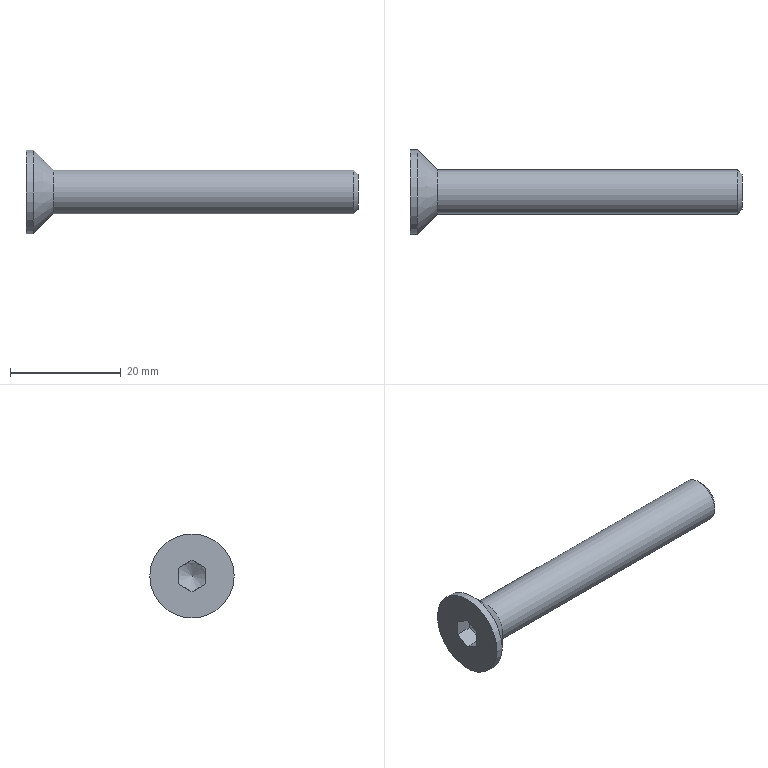Part | STEP file | DIN 7991 - M8  x  60 | 1 solid | 13 faces | box 60 x 15.24 x 15.24 mm | volume 3321 mm3 | plane 8 | cone 3 | cylinder 2 | commonest cylinder face diameters 8 x1 15.24 x1
STEP:
#1=CARTESIAN_POINT('',(0.,0.,0.));
#2=DIRECTION('',(0.,0.,1.));
#3=DIRECTION('',(1.,0.,0.));
#4=AXIS2_PLACEMENT_3D('',#1,#2,#3);
#5=CARTESIAN_POINT('',(59.233,4.,0.));
#6=VERTEX_POINT('',#5);
#7=CARTESIAN_POINT('',(59.233,0.,0.));
#8=DIRECTION('',(1.,0.,0.));
#9=DIRECTION('',(0.,-1.,0.));
#10=AXIS2_PLACEMENT_3D('',#7,#8,#9);
#11=CIRCLE('',#10,4.);
#12=CARTESIAN_POINT('',(59.617,0.,0.));
#13=DIRECTION('',(-1.,0.,0.));
#14=DIRECTION('',(0.,-1.,0.));
#15=AXIS2_PLACEMENT_3D('',#12,#13,#14);
#16=CONICAL_SURFACE('',#15,3.617,0.7854);
#17=CARTESIAN_POINT('',(12.566,0.3834));
#18=DIRECTION('',(-1.,0.));
#19=VECTOR('',#18,1.);
#20=LINE('',#17,#19);
#21=(GEOMETRIC_REPRESENTATION_CONTEXT(2)PARAMETRIC_REPRESENTATION_CONTEXT()REPRESENTATION_CONTEXT('',''));
#22=DEFINITIONAL_REPRESENTATION('',(#20),#21);
#23=PCURVE('',#16,#22);
#24=CARTESIAN_POINT('',(46.,0.,0.));
#25=DIRECTION('',(1.,0.,0.));
#26=DIRECTION('',(0.,1.,0.));
#27=AXIS2_PLACEMENT_3D('',#24,#25,#26);
#28=CYLINDRICAL_SURFACE('',#27,4.);
#29=CARTESIAN_POINT('',(-3.142,13.233));
#30=DIRECTION('',(1.,0.));
#31=VECTOR('',#30,1.);
#32=LINE('',#29,#31);
#33=(GEOMETRIC_REPRESENTATION_CONTEXT(2)PARAMETRIC_REPRESENTATION_CONTEXT()REPRESENTATION_CONTEXT('',''));
#34=DEFINITIONAL_REPRESENTATION('',(#32),#33);
#35=PCURVE('',#28,#34);
#36=SURFACE_CURVE('',#11,(#23,#35),.PCURVE_S1.);
#37=EDGE_CURVE('',#6,#6,#36,.T.);
#38=ORIENTED_EDGE('',*,*,#37,.T.);
#39=CARTESIAN_POINT('',(60.,3.233,0.));
#40=VERTEX_POINT('',#39);
#41=CARTESIAN_POINT('',(60.,3.233,0.));
#42=CARTESIAN_POINT('',(59.233,4.,0.));
#43=B_SPLINE_CURVE_WITH_KNOTS('',1,(#41,#42),.UNSPECIFIED.,.F.,.F.,(2,2),(-0.5422,0.5422),.PIECEWISE_BEZIER_KNOTS.);
#44=CARTESIAN_POINT('',(3.142,0.));
#45=DIRECTION('',(0.,1.));
#46=VECTOR('',#45,1.);
#47=LINE('',#44,#46);
#48=(GEOMETRIC_REPRESENTATION_CONTEXT(2)PARAMETRIC_REPRESENTATION_CONTEXT()REPRESENTATION_CONTEXT('',''));
#49=DEFINITIONAL_REPRESENTATION('',(#47),#48);
#50=PCURVE('',#16,#49);
#51=CARTESIAN_POINT('',(9.425,0.));
#52=DIRECTION('',(0.,1.));
#53=VECTOR('',#52,1.);
#54=LINE('',#51,#53);
#55=(GEOMETRIC_REPRESENTATION_CONTEXT(2)PARAMETRIC_REPRESENTATION_CONTEXT()REPRESENTATION_CONTEXT('',''));
#56=DEFINITIONAL_REPRESENTATION('',(#54),#55);
#57=PCURVE('',#16,#56);
#58=SEAM_CURVE('',#43,(#50,#57),.PCURVE_S1.);
#59=EDGE_CURVE('',#40,#6,#58,.T.);
#60=ORIENTED_EDGE('',*,*,#59,.F.);
#61=CARTESIAN_POINT('',(60.,0.,0.));
#62=DIRECTION('',(-1.,0.,0.));
#63=DIRECTION('',(0.,-1.,0.));
#64=AXIS2_PLACEMENT_3D('',#61,#62,#63);
#65=CIRCLE('',#64,3.233);
#66=CARTESIAN_POINT('',(0.,-0.3834));
#67=DIRECTION('',(1.,0.));
#68=VECTOR('',#67,1.);
#69=LINE('',#66,#68);
#70=(GEOMETRIC_REPRESENTATION_CONTEXT(2)PARAMETRIC_REPRESENTATION_CONTEXT()REPRESENTATION_CONTEXT('',''));
#71=DEFINITIONAL_REPRESENTATION('',(#69),#70);
#72=PCURVE('',#16,#71);
#73=CARTESIAN_POINT('',(60.,2.,0.));
#74=DIRECTION('',(1.,0.,0.));
#75=DIRECTION('',(0.,0.,-1.));
#76=AXIS2_PLACEMENT_3D('',#73,#74,#75);
#77=PLANE('',#76);
#78=CARTESIAN_POINT('',(0.,-5.233));
#79=CARTESIAN_POINT('',(-5.6,-5.233));
#80=CARTESIAN_POINT('',(-2.8,-0.3834));
#81=CARTESIAN_POINT('',(0.,4.466));
#82=CARTESIAN_POINT('',(2.8,-0.3834));
#83=CARTESIAN_POINT('',(5.6,-5.233));
#84=CARTESIAN_POINT('',(0.,-5.233));
#85=(BOUNDED_CURVE()B_SPLINE_CURVE(2,(#78,#79,#80,#81,#82,#83,#84),.UNSPECIFIED.,.T.,.F.)B_SPLINE_CURVE_WITH_KNOTS((1,2,2,2,2,1),(-2.094,0.,2.094,4.189,6.283,8.378),.UNSPECIFIED.)CURVE()GEOMETRIC_REPRESENTATION_ITEM()RATIONAL_B_SPLINE_CURVE((1.,0.5,1.,0.5,1.,0.5,1.))REPRESENTATION_ITEM(''));
#86=(GEOMETRIC_REPRESENTATION_CONTEXT(2)PARAMETRIC_REPRESENTATION_CONTEXT()REPRESENTATION_CONTEXT('',''));
#87=DEFINITIONAL_REPRESENTATION('',(#85),#86);
#88=PCURVE('',#77,#87);
#89=SURFACE_CURVE('',#65,(#72,#88),.PCURVE_S1.);
#90=EDGE_CURVE('',#40,#40,#89,.T.);
#91=ORIENTED_EDGE('',*,*,#90,.T.);
#92=ORIENTED_EDGE('',*,*,#59,.T.);
#93=EDGE_LOOP('',(#38,#60,#91,#92));
#94=FACE_BOUND('',#93,.T.);
#95=ADVANCED_FACE('',(#94),#16,.T.);
#96=CARTESIAN_POINT('',(4.96,4.,0.));
#97=VERTEX_POINT('',#96);
#98=CARTESIAN_POINT('',(4.96,0.,0.));
#99=DIRECTION('',(1.,0.,0.));
#100=DIRECTION('',(0.,1.,0.));
#101=AXIS2_PLACEMENT_3D('',#98,#99,#100);
#102=CIRCLE('',#101,4.);
#103=CARTESIAN_POINT('',(0.,-41.04));
#104=DIRECTION('',(1.,0.));
#105=VECTOR('',#104,1.);
#106=LINE('',#103,#105);
#107=(GEOMETRIC_REPRESENTATION_CONTEXT(2)PARAMETRIC_REPRESENTATION_CONTEXT()REPRESENTATION_CONTEXT('',''));
#108=DEFINITIONAL_REPRESENTATION('',(#106),#107);
#109=PCURVE('',#28,#108);
#110=CARTESIAN_POINT('',(3.15,0.,0.));
#111=DIRECTION('',(-1.,0.,0.));
#112=DIRECTION('',(0.,1.,0.));
#113=AXIS2_PLACEMENT_3D('',#110,#111,#112);
#114=CONICAL_SURFACE('',#113,5.81,0.7854);
#115=CARTESIAN_POINT('',(6.283,-1.81));
#116=DIRECTION('',(-1.,0.));
#117=VECTOR('',#116,1.);
#118=LINE('',#115,#117);
#119=(GEOMETRIC_REPRESENTATION_CONTEXT(2)PARAMETRIC_REPRESENTATION_CONTEXT()REPRESENTATION_CONTEXT('',''));
#120=DEFINITIONAL_REPRESENTATION('',(#118),#119);
#121=PCURVE('',#114,#120);
#122=SURFACE_CURVE('',#102,(#109,#121),.PCURVE_S1.);
#123=EDGE_CURVE('',#97,#97,#122,.T.);
#124=ORIENTED_EDGE('',*,*,#123,.T.);
#125=CARTESIAN_POINT('',(4.96,4.,0.));
#126=CARTESIAN_POINT('',(59.233,4.,0.));
#127=B_SPLINE_CURVE_WITH_KNOTS('',1,(#125,#126),.UNSPECIFIED.,.F.,.F.,(2,2),(-41.04,13.233),.PIECEWISE_BEZIER_KNOTS.);
#128=CARTESIAN_POINT('',(6.283,0.));
#129=DIRECTION('',(0.,1.));
#130=VECTOR('',#129,1.);
#131=LINE('',#128,#130);
#132=(GEOMETRIC_REPRESENTATION_CONTEXT(2)PARAMETRIC_REPRESENTATION_CONTEXT()REPRESENTATION_CONTEXT('',''));
#133=DEFINITIONAL_REPRESENTATION('',(#131),#132);
#134=PCURVE('',#28,#133);
#135=CARTESIAN_POINT('',(0.,0.));
#136=DIRECTION('',(0.,1.));
#137=VECTOR('',#136,1.);
#138=LINE('',#135,#137);
#139=(GEOMETRIC_REPRESENTATION_CONTEXT(2)PARAMETRIC_REPRESENTATION_CONTEXT()REPRESENTATION_CONTEXT('',''));
#140=DEFINITIONAL_REPRESENTATION('',(#138),#139);
#141=PCURVE('',#28,#140);
#142=SEAM_CURVE('',#127,(#134,#141),.PCURVE_S1.);
#143=EDGE_CURVE('',#97,#6,#142,.T.);
#144=ORIENTED_EDGE('',*,*,#143,.T.);
#145=ORIENTED_EDGE('',*,*,#37,.F.);
#146=ORIENTED_EDGE('',*,*,#143,.F.);
#147=EDGE_LOOP('',(#124,#144,#145,#146));
#148=FACE_BOUND('',#147,.T.);
#149=ADVANCED_FACE('',(#148),#28,.T.);
#150=ORIENTED_EDGE('',*,*,#90,.F.);
#151=EDGE_LOOP('',(#150));
#152=FACE_BOUND('',#151,.T.);
#153=ADVANCED_FACE('',(#152),#77,.T.);
#154=CARTESIAN_POINT('',(3.,-2.5,-1.443));
#155=VERTEX_POINT('',#154);
#156=CARTESIAN_POINT('',(3.,-2.5,1.443));
#157=VERTEX_POINT('',#156);
#158=CARTESIAN_POINT('',(3.,-2.5,-1.443));
#159=CARTESIAN_POINT('',(3.417,-2.5,0.));
#160=CARTESIAN_POINT('',(3.,-2.5,1.443));
#161=(BOUNDED_CURVE()B_SPLINE_CURVE(2,(#158,#159,#160),.UNSPECIFIED.,.F.,.F.)B_SPLINE_CURVE_WITH_KNOTS((3,3),(0.,0.2921),.PIECEWISE_BEZIER_KNOTS.)CURVE()GEOMETRIC_REPRESENTATION_ITEM()RATIONAL_B_SPLINE_CURVE((1.,1.155,1.))REPRESENTATION_ITEM(''));
#162=CARTESIAN_POINT('',(0.,-2.5,-1.443));
#163=DIRECTION('',(0.,-1.,0.));
#164=DIRECTION('',(0.,0.,-1.));
#165=AXIS2_PLACEMENT_3D('',#162,#163,#164);
#166=PLANE('',#165);
#167=CARTESIAN_POINT('',(0.,3.));
#168=CARTESIAN_POINT('',(-1.443,3.417));
#169=CARTESIAN_POINT('',(-2.887,3.));
#170=(BOUNDED_CURVE()B_SPLINE_CURVE(2,(#167,#168,#169),.UNSPECIFIED.,.F.,.F.)B_SPLINE_CURVE_WITH_KNOTS((3,3),(0.,0.2921),.PIECEWISE_BEZIER_KNOTS.)CURVE()GEOMETRIC_REPRESENTATION_ITEM()RATIONAL_B_SPLINE_CURVE((1.,1.155,1.))REPRESENTATION_ITEM(''));
#171=(GEOMETRIC_REPRESENTATION_CONTEXT(2)PARAMETRIC_REPRESENTATION_CONTEXT()REPRESENTATION_CONTEXT('',''));
#172=DEFINITIONAL_REPRESENTATION('',(#170),#171);
#173=PCURVE('',#166,#172);
#174=CARTESIAN_POINT('',(3.833,0.,0.));
#175=DIRECTION('',(-1.,0.,0.));
#176=DIRECTION('',(0.,1.,0.));
#177=AXIS2_PLACEMENT_3D('',#174,#175,#176);
#178=CONICAL_SURFACE('',#177,1.443,1.047);
#179=CARTESIAN_POINT('',(8.901,0.8333));
#180=CARTESIAN_POINT('',(8.916,0.8188));
#181=CARTESIAN_POINT('',(8.947,0.7913));
#182=CARTESIAN_POINT('',(8.993,0.755));
#183=CARTESIAN_POINT('',(9.04,0.7233));
#184=CARTESIAN_POINT('',(9.087,0.6958));
#185=CARTESIAN_POINT('',(9.134,0.6724));
#186=CARTESIAN_POINT('',(9.182,0.6529));
#187=CARTESIAN_POINT('',(9.23,0.6371));
#188=CARTESIAN_POINT('',(9.279,0.625));
#189=CARTESIAN_POINT('',(9.327,0.6163));
#190=CARTESIAN_POINT('',(9.376,0.6112));
#191=CARTESIAN_POINT('',(9.425,0.6095));
#192=CARTESIAN_POINT('',(9.473,0.6112));
#193=CARTESIAN_POINT('',(9.522,0.6163));
#194=CARTESIAN_POINT('',(9.571,0.625));
#195=CARTESIAN_POINT('',(9.619,0.6371));
#196=CARTESIAN_POINT('',(9.667,0.6529));
#197=CARTESIAN_POINT('',(9.715,0.6724));
#198=CARTESIAN_POINT('',(9.763,0.6958));
#199=CARTESIAN_POINT('',(9.81,0.7233));
#200=CARTESIAN_POINT('',(9.856,0.755));
#201=CARTESIAN_POINT('',(9.903,0.7913));
#202=CARTESIAN_POINT('',(9.933,0.8188));
#203=CARTESIAN_POINT('',(9.948,0.8333));
#204=B_SPLINE_CURVE_WITH_KNOTS('',3,(#179,#180,#181,#182,#183,#184,#185,#186,#187,#188,#189,#190,#191,#192,#193,#194,#195,#196,#197,#198,#199,#200,#201,#202,#203),.UNSPECIFIED.,.F.,.F.,(4,1,1,1,1,1,1,1,1,1,1,1,1,1,1,1,1,1,1,1,1,1,4),(0.,0.01328,0.02656,0.03983,0.05311,0.06639,0.07967,0.09294,0.1062,0.1195,0.1328,0.1461,0.1593,0.1726,0.1859,0.1992,0.2124,0.2257,0.239,0.2523,0.2656,0.2788,0.2921),.QUASI_UNIFORM_KNOTS.);
#205=(GEOMETRIC_REPRESENTATION_CONTEXT(2)PARAMETRIC_REPRESENTATION_CONTEXT()REPRESENTATION_CONTEXT('',''));
#206=DEFINITIONAL_REPRESENTATION('',(#204),#205);
#207=PCURVE('',#178,#206);
#208=SURFACE_CURVE('',#161,(#173,#207),.PCURVE_S1.);
#209=EDGE_CURVE('',#155,#157,#208,.T.);
#210=ORIENTED_EDGE('',*,*,#209,.F.);
#211=CARTESIAN_POINT('',(0.,-2.5,-1.443));
#212=VERTEX_POINT('',#211);
#213=CARTESIAN_POINT('',(1.5,-2.5,-1.443));
#214=DIRECTION('',(-1.,0.,0.));
#215=VECTOR('',#214,1.);
#216=LINE('',#213,#215);
#217=CARTESIAN_POINT('',(0.,1.5));
#218=DIRECTION('',(0.,-1.));
#219=VECTOR('',#218,1.);
#220=LINE('',#217,#219);
#221=(GEOMETRIC_REPRESENTATION_CONTEXT(2)PARAMETRIC_REPRESENTATION_CONTEXT()REPRESENTATION_CONTEXT('',''));
#222=DEFINITIONAL_REPRESENTATION('',(#220),#221);
#223=PCURVE('',#166,#222);
#224=CARTESIAN_POINT('',(0.,0.,-2.887));
#225=DIRECTION('',(0.,-0.5,-0.866));
#226=DIRECTION('',(-1.,0.,0.));
#227=AXIS2_PLACEMENT_3D('',#224,#225,#226);
#228=PLANE('',#227);
#229=CARTESIAN_POINT('',(-1.5,-2.887));
#230=DIRECTION('',(1.,0.));
#231=VECTOR('',#230,1.);
#232=LINE('',#229,#231);
#233=(GEOMETRIC_REPRESENTATION_CONTEXT(2)PARAMETRIC_REPRESENTATION_CONTEXT()REPRESENTATION_CONTEXT('',''));
#234=DEFINITIONAL_REPRESENTATION('',(#232),#233);
#235=PCURVE('',#228,#234);
#236=SURFACE_CURVE('',#216,(#223,#235),.PCURVE_S1.);
#237=EDGE_CURVE('',#155,#212,#236,.T.);
#238=ORIENTED_EDGE('',*,*,#237,.T.);
#239=CARTESIAN_POINT('',(0.,-2.5,1.443));
#240=VERTEX_POINT('',#239);
#241=CARTESIAN_POINT('',(0.,-2.5,-0.6526));
#242=DIRECTION('',(0.,0.,-1.));
#243=VECTOR('',#242,1.);
#244=LINE('',#241,#243);
#245=CARTESIAN_POINT('',(-0.7907,0.));
#246=DIRECTION('',(1.,0.));
#247=VECTOR('',#246,1.);
#248=LINE('',#245,#247);
#249=(GEOMETRIC_REPRESENTATION_CONTEXT(2)PARAMETRIC_REPRESENTATION_CONTEXT()REPRESENTATION_CONTEXT('',''));
#250=DEFINITIONAL_REPRESENTATION('',(#248),#249);
#251=PCURVE('',#166,#250);
#252=CARTESIAN_POINT('',(0.,5.253,0.));
#253=DIRECTION('',(-1.,0.,0.));
#254=DIRECTION('',(0.,0.,1.));
#255=AXIS2_PLACEMENT_3D('',#252,#253,#254);
#256=PLANE('',#255);
#257=CARTESIAN_POINT('',(-0.6526,-7.753));
#258=DIRECTION('',(-1.,0.));
#259=VECTOR('',#258,1.);
#260=LINE('',#257,#259);
#261=(GEOMETRIC_REPRESENTATION_CONTEXT(2)PARAMETRIC_REPRESENTATION_CONTEXT()REPRESENTATION_CONTEXT('',''));
#262=DEFINITIONAL_REPRESENTATION('',(#260),#261);
#263=PCURVE('',#256,#262);
#264=SURFACE_CURVE('',#244,(#251,#263),.PCURVE_S1.);
#265=EDGE_CURVE('',#240,#212,#264,.T.);
#266=ORIENTED_EDGE('',*,*,#265,.F.);
#267=CARTESIAN_POINT('',(1.5,-2.5,1.443));
#268=DIRECTION('',(-1.,0.,0.));
#269=VECTOR('',#268,1.);
#270=LINE('',#267,#269);
#271=CARTESIAN_POINT('',(-2.887,1.5));
#272=DIRECTION('',(0.,-1.));
#273=VECTOR('',#272,1.);
#274=LINE('',#271,#273);
#275=(GEOMETRIC_REPRESENTATION_CONTEXT(2)PARAMETRIC_REPRESENTATION_CONTEXT()REPRESENTATION_CONTEXT('',''));
#276=DEFINITIONAL_REPRESENTATION('',(#274),#275);
#277=PCURVE('',#166,#276);
#278=CARTESIAN_POINT('',(0.,-2.5,1.443));
#279=DIRECTION('',(0.,-0.5,0.866));
#280=DIRECTION('',(1.,0.,0.));
#281=AXIS2_PLACEMENT_3D('',#278,#279,#280);
#282=PLANE('',#281);
#283=CARTESIAN_POINT('',(1.5,0.));
#284=DIRECTION('',(-1.,0.));
#285=VECTOR('',#284,1.);
#286=LINE('',#283,#285);
#287=(GEOMETRIC_REPRESENTATION_CONTEXT(2)PARAMETRIC_REPRESENTATION_CONTEXT()REPRESENTATION_CONTEXT('',''));
#288=DEFINITIONAL_REPRESENTATION('',(#286),#287);
#289=PCURVE('',#282,#288);
#290=SURFACE_CURVE('',#270,(#277,#289),.PCURVE_S1.);
#291=EDGE_CURVE('',#157,#240,#290,.T.);
#292=ORIENTED_EDGE('',*,*,#291,.F.);
#293=EDGE_LOOP('',(#210,#238,#266,#292));
#294=FACE_BOUND('',#293,.T.);
#295=ADVANCED_FACE('',(#294),#166,.F.);
#296=CARTESIAN_POINT('',(3.,0.,-2.887));
#297=VERTEX_POINT('',#296);
#298=CARTESIAN_POINT('',(3.,0.,-2.887));
#299=CARTESIAN_POINT('',(3.417,-1.25,-2.165));
#300=CARTESIAN_POINT('',(3.,-2.5,-1.443));
#301=(BOUNDED_CURVE()B_SPLINE_CURVE(2,(#298,#299,#300),.UNSPECIFIED.,.F.,.F.)B_SPLINE_CURVE_WITH_KNOTS((3,3),(0.,0.2921),.PIECEWISE_BEZIER_KNOTS.)CURVE()GEOMETRIC_REPRESENTATION_ITEM()RATIONAL_B_SPLINE_CURVE((1.,1.155,1.))REPRESENTATION_ITEM(''));
#302=CARTESIAN_POINT('',(-3.,0.));
#303=CARTESIAN_POINT('',(-3.417,-1.443));
#304=CARTESIAN_POINT('',(-3.,-2.887));
#305=(BOUNDED_CURVE()B_SPLINE_CURVE(2,(#302,#303,#304),.UNSPECIFIED.,.F.,.F.)B_SPLINE_CURVE_WITH_KNOTS((3,3),(0.,0.2921),.PIECEWISE_BEZIER_KNOTS.)CURVE()GEOMETRIC_REPRESENTATION_ITEM()RATIONAL_B_SPLINE_CURVE((1.,1.155,1.))REPRESENTATION_ITEM(''));
#306=(GEOMETRIC_REPRESENTATION_CONTEXT(2)PARAMETRIC_REPRESENTATION_CONTEXT()REPRESENTATION_CONTEXT('',''));
#307=DEFINITIONAL_REPRESENTATION('',(#305),#306);
#308=PCURVE('',#228,#307);
#309=CARTESIAN_POINT('',(7.854,0.8333));
#310=CARTESIAN_POINT('',(7.869,0.8188));
#311=CARTESIAN_POINT('',(7.9,0.7913));
#312=CARTESIAN_POINT('',(7.946,0.755));
#313=CARTESIAN_POINT('',(7.993,0.7233));
#314=CARTESIAN_POINT('',(8.04,0.6958));
#315=CARTESIAN_POINT('',(8.087,0.6724));
#316=CARTESIAN_POINT('',(8.135,0.6529));
#317=CARTESIAN_POINT('',(8.183,0.6371));
#318=CARTESIAN_POINT('',(8.232,0.625));
#319=CARTESIAN_POINT('',(8.28,0.6163));
#320=CARTESIAN_POINT('',(8.329,0.6112));
#321=CARTESIAN_POINT('',(8.378,0.6095));
#322=CARTESIAN_POINT('',(8.426,0.6112));
#323=CARTESIAN_POINT('',(8.475,0.6163));
#324=CARTESIAN_POINT('',(8.524,0.625));
#325=CARTESIAN_POINT('',(8.572,0.6371));
#326=CARTESIAN_POINT('',(8.62,0.6529));
#327=CARTESIAN_POINT('',(8.668,0.6724));
#328=CARTESIAN_POINT('',(8.715,0.6958));
#329=CARTESIAN_POINT('',(8.763,0.7233));
#330=CARTESIAN_POINT('',(8.809,0.755));
#331=CARTESIAN_POINT('',(8.856,0.7913));
#332=CARTESIAN_POINT('',(8.886,0.8188));
#333=CARTESIAN_POINT('',(8.901,0.8333));
#334=B_SPLINE_CURVE_WITH_KNOTS('',3,(#309,#310,#311,#312,#313,#314,#315,#316,#317,#318,#319,#320,#321,#322,#323,#324,#325,#326,#327,#328,#329,#330,#331,#332,#333),.UNSPECIFIED.,.F.,.F.,(4,1,1,1,1,1,1,1,1,1,1,1,1,1,1,1,1,1,1,1,1,1,4),(0.,0.01328,0.02656,0.03983,0.05311,0.06639,0.07967,0.09294,0.1062,0.1195,0.1328,0.1461,0.1593,0.1726,0.1859,0.1992,0.2124,0.2257,0.239,0.2523,0.2656,0.2788,0.2921),.QUASI_UNIFORM_KNOTS.);
#335=(GEOMETRIC_REPRESENTATION_CONTEXT(2)PARAMETRIC_REPRESENTATION_CONTEXT()REPRESENTATION_CONTEXT('',''));
#336=DEFINITIONAL_REPRESENTATION('',(#334),#335);
#337=PCURVE('',#178,#336);
#338=SURFACE_CURVE('',#301,(#308,#337),.PCURVE_S1.);
#339=EDGE_CURVE('',#297,#155,#338,.T.);
#340=ORIENTED_EDGE('',*,*,#339,.F.);
#341=CARTESIAN_POINT('',(0.,0.,-2.887));
#342=VERTEX_POINT('',#341);
#343=CARTESIAN_POINT('',(1.5,0.,-2.887));
#344=DIRECTION('',(-1.,0.,0.));
#345=VECTOR('',#344,1.);
#346=LINE('',#343,#345);
#347=CARTESIAN_POINT('',(-1.5,0.));
#348=DIRECTION('',(1.,0.));
#349=VECTOR('',#348,1.);
#350=LINE('',#347,#349);
#351=(GEOMETRIC_REPRESENTATION_CONTEXT(2)PARAMETRIC_REPRESENTATION_CONTEXT()REPRESENTATION_CONTEXT('',''));
#352=DEFINITIONAL_REPRESENTATION('',(#350),#351);
#353=PCURVE('',#228,#352);
#354=CARTESIAN_POINT('',(0.,2.5,-1.443));
#355=DIRECTION('',(0.,0.5,-0.866));
#356=DIRECTION('',(-1.,0.,0.));
#357=AXIS2_PLACEMENT_3D('',#354,#355,#356);
#358=PLANE('',#357);
#359=CARTESIAN_POINT('',(-1.5,-2.887));
#360=DIRECTION('',(1.,0.));
#361=VECTOR('',#360,1.);
#362=LINE('',#359,#361);
#363=(GEOMETRIC_REPRESENTATION_CONTEXT(2)PARAMETRIC_REPRESENTATION_CONTEXT()REPRESENTATION_CONTEXT('',''));
#364=DEFINITIONAL_REPRESENTATION('',(#362),#363);
#365=PCURVE('',#358,#364);
#366=SURFACE_CURVE('',#346,(#353,#365),.PCURVE_S1.);
#367=EDGE_CURVE('',#297,#342,#366,.T.);
#368=ORIENTED_EDGE('',*,*,#367,.T.);
#369=CARTESIAN_POINT('',(0.,-0.6031,-2.539));
#370=DIRECTION('',(0.,0.866,-0.5));
#371=VECTOR('',#370,1.);
#372=LINE('',#369,#371);
#373=CARTESIAN_POINT('',(0.,-0.6964));
#374=DIRECTION('',(0.,1.));
#375=VECTOR('',#374,1.);
#376=LINE('',#373,#375);
#377=(GEOMETRIC_REPRESENTATION_CONTEXT(2)PARAMETRIC_REPRESENTATION_CONTEXT()REPRESENTATION_CONTEXT('',''));
#378=DEFINITIONAL_REPRESENTATION('',(#376),#377);
#379=PCURVE('',#228,#378);
#380=CARTESIAN_POINT('',(-2.539,-5.856));
#381=DIRECTION('',(-0.5,0.866));
#382=VECTOR('',#381,1.);
#383=LINE('',#380,#382);
#384=(GEOMETRIC_REPRESENTATION_CONTEXT(2)PARAMETRIC_REPRESENTATION_CONTEXT()REPRESENTATION_CONTEXT('',''));
#385=DEFINITIONAL_REPRESENTATION('',(#383),#384);
#386=PCURVE('',#256,#385);
#387=SURFACE_CURVE('',#372,(#379,#386),.PCURVE_S1.);
#388=EDGE_CURVE('',#212,#342,#387,.T.);
#389=ORIENTED_EDGE('',*,*,#388,.F.);
#390=ORIENTED_EDGE('',*,*,#237,.F.);
#391=EDGE_LOOP('',(#340,#368,#389,#390));
#392=FACE_BOUND('',#391,.T.);
#393=ADVANCED_FACE('',(#392),#228,.F.);
#394=CARTESIAN_POINT('',(3.,2.5,-1.443));
#395=VERTEX_POINT('',#394);
#396=CARTESIAN_POINT('',(3.,2.5,-1.443));
#397=CARTESIAN_POINT('',(3.417,1.25,-2.165));
#398=CARTESIAN_POINT('',(3.,0.,-2.887));
#399=(BOUNDED_CURVE()B_SPLINE_CURVE(2,(#396,#397,#398),.UNSPECIFIED.,.F.,.F.)B_SPLINE_CURVE_WITH_KNOTS((3,3),(0.,0.2921),.PIECEWISE_BEZIER_KNOTS.)CURVE()GEOMETRIC_REPRESENTATION_ITEM()RATIONAL_B_SPLINE_CURVE((1.,1.155,1.))REPRESENTATION_ITEM(''));
#400=CARTESIAN_POINT('',(-3.,0.));
#401=CARTESIAN_POINT('',(-3.417,-1.443));
#402=CARTESIAN_POINT('',(-3.,-2.887));
#403=(BOUNDED_CURVE()B_SPLINE_CURVE(2,(#400,#401,#402),.UNSPECIFIED.,.F.,.F.)B_SPLINE_CURVE_WITH_KNOTS((3,3),(0.,0.2921),.PIECEWISE_BEZIER_KNOTS.)CURVE()GEOMETRIC_REPRESENTATION_ITEM()RATIONAL_B_SPLINE_CURVE((1.,1.155,1.))REPRESENTATION_ITEM(''));
#404=(GEOMETRIC_REPRESENTATION_CONTEXT(2)PARAMETRIC_REPRESENTATION_CONTEXT()REPRESENTATION_CONTEXT('',''));
#405=DEFINITIONAL_REPRESENTATION('',(#403),#404);
#406=PCURVE('',#358,#405);
#407=CARTESIAN_POINT('',(6.807,0.8333));
#408=CARTESIAN_POINT('',(6.822,0.8188));
#409=CARTESIAN_POINT('',(6.852,0.7913));
#410=CARTESIAN_POINT('',(6.899,0.755));
#411=CARTESIAN_POINT('',(6.945,0.7233));
#412=CARTESIAN_POINT('',(6.993,0.6958));
#413=CARTESIAN_POINT('',(7.04,0.6724));
#414=CARTESIAN_POINT('',(7.088,0.6529));
#415=CARTESIAN_POINT('',(7.136,0.6371));
#416=CARTESIAN_POINT('',(7.184,0.625));
#417=CARTESIAN_POINT('',(7.233,0.6163));
#418=CARTESIAN_POINT('',(7.282,0.6112));
#419=CARTESIAN_POINT('',(7.33,0.6095));
#420=CARTESIAN_POINT('',(7.379,0.6112));
#421=CARTESIAN_POINT('',(7.428,0.6163));
#422=CARTESIAN_POINT('',(7.476,0.625));
#423=CARTESIAN_POINT('',(7.525,0.6371));
#424=CARTESIAN_POINT('',(7.573,0.6529));
#425=CARTESIAN_POINT('',(7.621,0.6724));
#426=CARTESIAN_POINT('',(7.668,0.6958));
#427=CARTESIAN_POINT('',(7.715,0.7233));
#428=CARTESIAN_POINT('',(7.762,0.755));
#429=CARTESIAN_POINT('',(7.808,0.7913));
#430=CARTESIAN_POINT('',(7.839,0.8188));
#431=CARTESIAN_POINT('',(7.854,0.8333));
#432=B_SPLINE_CURVE_WITH_KNOTS('',3,(#407,#408,#409,#410,#411,#412,#413,#414,#415,#416,#417,#418,#419,#420,#421,#422,#423,#424,#425,#426,#427,#428,#429,#430,#431),.UNSPECIFIED.,.F.,.F.,(4,1,1,1,1,1,1,1,1,1,1,1,1,1,1,1,1,1,1,1,1,1,4),(0.,0.01328,0.02656,0.03983,0.05311,0.06639,0.07967,0.09294,0.1062,0.1195,0.1328,0.1461,0.1593,0.1726,0.1859,0.1992,0.2124,0.2257,0.239,0.2523,0.2656,0.2788,0.2921),.QUASI_UNIFORM_KNOTS.);
#433=(GEOMETRIC_REPRESENTATION_CONTEXT(2)PARAMETRIC_REPRESENTATION_CONTEXT()REPRESENTATION_CONTEXT('',''));
#434=DEFINITIONAL_REPRESENTATION('',(#432),#433);
#435=PCURVE('',#178,#434);
#436=SURFACE_CURVE('',#399,(#406,#435),.PCURVE_S1.);
#437=EDGE_CURVE('',#395,#297,#436,.T.);
#438=ORIENTED_EDGE('',*,*,#437,.F.);
#439=CARTESIAN_POINT('',(0.,2.5,-1.443));
#440=VERTEX_POINT('',#439);
#441=CARTESIAN_POINT('',(1.5,2.5,-1.443));
#442=DIRECTION('',(-1.,0.,0.));
#443=VECTOR('',#442,1.);
#444=LINE('',#441,#443);
#445=CARTESIAN_POINT('',(-1.5,0.));
#446=DIRECTION('',(1.,0.));
#447=VECTOR('',#446,1.);
#448=LINE('',#445,#447);
#449=(GEOMETRIC_REPRESENTATION_CONTEXT(2)PARAMETRIC_REPRESENTATION_CONTEXT()REPRESENTATION_CONTEXT('',''));
#450=DEFINITIONAL_REPRESENTATION('',(#448),#449);
#451=PCURVE('',#358,#450);
#452=CARTESIAN_POINT('',(0.,2.5,1.443));
#453=DIRECTION('',(0.,1.,0.));
#454=DIRECTION('',(0.,0.,1.));
#455=AXIS2_PLACEMENT_3D('',#452,#453,#454);
#456=PLANE('',#455);
#457=CARTESIAN_POINT('',(-2.887,1.5));
#458=DIRECTION('',(0.,-1.));
#459=VECTOR('',#458,1.);
#460=LINE('',#457,#459);
#461=(GEOMETRIC_REPRESENTATION_CONTEXT(2)PARAMETRIC_REPRESENTATION_CONTEXT()REPRESENTATION_CONTEXT('',''));
#462=DEFINITIONAL_REPRESENTATION('',(#460),#461);
#463=PCURVE('',#456,#462);
#464=SURFACE_CURVE('',#444,(#451,#463),.PCURVE_S1.);
#465=EDGE_CURVE('',#395,#440,#464,.T.);
#466=ORIENTED_EDGE('',*,*,#465,.T.);
#467=CARTESIAN_POINT('',(0.,1.957,-1.757));
#468=DIRECTION('',(0.,0.866,0.5));
#469=VECTOR('',#468,1.);
#470=LINE('',#467,#469);
#471=CARTESIAN_POINT('',(0.,-0.6274));
#472=DIRECTION('',(0.,1.));
#473=VECTOR('',#472,1.);
#474=LINE('',#471,#473);
#475=(GEOMETRIC_REPRESENTATION_CONTEXT(2)PARAMETRIC_REPRESENTATION_CONTEXT()REPRESENTATION_CONTEXT('',''));
#476=DEFINITIONAL_REPRESENTATION('',(#474),#475);
#477=PCURVE('',#358,#476);
#478=CARTESIAN_POINT('',(-1.757,-3.297));
#479=DIRECTION('',(0.5,0.866));
#480=VECTOR('',#479,1.);
#481=LINE('',#478,#480);
#482=(GEOMETRIC_REPRESENTATION_CONTEXT(2)PARAMETRIC_REPRESENTATION_CONTEXT()REPRESENTATION_CONTEXT('',''));
#483=DEFINITIONAL_REPRESENTATION('',(#481),#482);
#484=PCURVE('',#256,#483);
#485=SURFACE_CURVE('',#470,(#477,#484),.PCURVE_S1.);
#486=EDGE_CURVE('',#342,#440,#485,.T.);
#487=ORIENTED_EDGE('',*,*,#486,.F.);
#488=ORIENTED_EDGE('',*,*,#367,.F.);
#489=EDGE_LOOP('',(#438,#466,#487,#488));
#490=FACE_BOUND('',#489,.T.);
#491=ADVANCED_FACE('',(#490),#358,.F.);
#492=CARTESIAN_POINT('',(3.,2.5,1.443));
#493=VERTEX_POINT('',#492);
#494=CARTESIAN_POINT('',(3.,2.5,1.443));
#495=CARTESIAN_POINT('',(3.417,2.5,0.));
#496=CARTESIAN_POINT('',(3.,2.5,-1.443));
#497=(BOUNDED_CURVE()B_SPLINE_CURVE(2,(#494,#495,#496),.UNSPECIFIED.,.F.,.F.)B_SPLINE_CURVE_WITH_KNOTS((3,3),(0.,0.2921),.PIECEWISE_BEZIER_KNOTS.)CURVE()GEOMETRIC_REPRESENTATION_ITEM()RATIONAL_B_SPLINE_CURVE((1.,1.155,1.))REPRESENTATION_ITEM(''));
#498=CARTESIAN_POINT('',(0.,3.));
#499=CARTESIAN_POINT('',(-1.443,3.417));
#500=CARTESIAN_POINT('',(-2.887,3.));
#501=(BOUNDED_CURVE()B_SPLINE_CURVE(2,(#498,#499,#500),.UNSPECIFIED.,.F.,.F.)B_SPLINE_CURVE_WITH_KNOTS((3,3),(0.,0.2921),.PIECEWISE_BEZIER_KNOTS.)CURVE()GEOMETRIC_REPRESENTATION_ITEM()RATIONAL_B_SPLINE_CURVE((1.,1.155,1.))REPRESENTATION_ITEM(''));
#502=(GEOMETRIC_REPRESENTATION_CONTEXT(2)PARAMETRIC_REPRESENTATION_CONTEXT()REPRESENTATION_CONTEXT('',''));
#503=DEFINITIONAL_REPRESENTATION('',(#501),#502);
#504=PCURVE('',#456,#503);
#505=CARTESIAN_POINT('',(5.76,0.8333));
#506=CARTESIAN_POINT('',(5.775,0.8188));
#507=CARTESIAN_POINT('',(5.805,0.7913));
#508=CARTESIAN_POINT('',(5.851,0.755));
#509=CARTESIAN_POINT('',(5.898,0.7233));
#510=CARTESIAN_POINT('',(5.945,0.6958));
#511=CARTESIAN_POINT('',(5.993,0.6724));
#512=CARTESIAN_POINT('',(6.041,0.6529));
#513=CARTESIAN_POINT('',(6.089,0.6371));
#514=CARTESIAN_POINT('',(6.137,0.625));
#515=CARTESIAN_POINT('',(6.186,0.6163));
#516=CARTESIAN_POINT('',(6.234,0.6112));
#517=CARTESIAN_POINT('',(6.283,0.6095));
#518=CARTESIAN_POINT('',(6.332,0.6112));
#519=CARTESIAN_POINT('',(6.381,0.6163));
#520=CARTESIAN_POINT('',(6.429,0.625));
#521=CARTESIAN_POINT('',(6.477,0.6371));
#522=CARTESIAN_POINT('',(6.526,0.6529));
#523=CARTESIAN_POINT('',(6.573,0.6724));
#524=CARTESIAN_POINT('',(6.621,0.6958));
#525=CARTESIAN_POINT('',(6.668,0.7233));
#526=CARTESIAN_POINT('',(6.715,0.755));
#527=CARTESIAN_POINT('',(6.761,0.7913));
#528=CARTESIAN_POINT('',(6.792,0.8188));
#529=CARTESIAN_POINT('',(6.807,0.8333));
#530=B_SPLINE_CURVE_WITH_KNOTS('',3,(#505,#506,#507,#508,#509,#510,#511,#512,#513,#514,#515,#516,#517,#518,#519,#520,#521,#522,#523,#524,#525,#526,#527,#528,#529),.UNSPECIFIED.,.F.,.F.,(4,1,1,1,1,1,1,1,1,1,1,1,1,1,1,1,1,1,1,1,1,1,4),(0.,0.01328,0.02656,0.03983,0.05311,0.06639,0.07967,0.09294,0.1062,0.1195,0.1328,0.1461,0.1593,0.1726,0.1859,0.1992,0.2124,0.2257,0.239,0.2523,0.2656,0.2788,0.2921),.QUASI_UNIFORM_KNOTS.);
#531=(GEOMETRIC_REPRESENTATION_CONTEXT(2)PARAMETRIC_REPRESENTATION_CONTEXT()REPRESENTATION_CONTEXT('',''));
#532=DEFINITIONAL_REPRESENTATION('',(#530),#531);
#533=PCURVE('',#178,#532);
#534=SURFACE_CURVE('',#497,(#504,#533),.PCURVE_S1.);
#535=EDGE_CURVE('',#493,#395,#534,.T.);
#536=ORIENTED_EDGE('',*,*,#535,.F.);
#537=CARTESIAN_POINT('',(0.,2.5,1.443));
#538=VERTEX_POINT('',#537);
#539=CARTESIAN_POINT('',(1.5,2.5,1.443));
#540=DIRECTION('',(1.,0.,0.));
#541=VECTOR('',#540,1.);
#542=LINE('',#539,#541);
#543=CARTESIAN_POINT('',(0.,1.5));
#544=DIRECTION('',(0.,1.));
#545=VECTOR('',#544,1.);
#546=LINE('',#543,#545);
#547=(GEOMETRIC_REPRESENTATION_CONTEXT(2)PARAMETRIC_REPRESENTATION_CONTEXT()REPRESENTATION_CONTEXT('',''));
#548=DEFINITIONAL_REPRESENTATION('',(#546),#547);
#549=PCURVE('',#456,#548);
#550=CARTESIAN_POINT('',(0.,0.,2.887));
#551=DIRECTION('',(0.,0.5,0.866));
#552=DIRECTION('',(1.,0.,0.));
#553=AXIS2_PLACEMENT_3D('',#550,#551,#552);
#554=PLANE('',#553);
#555=CARTESIAN_POINT('',(1.5,2.887));
#556=DIRECTION('',(1.,0.));
#557=VECTOR('',#556,1.);
#558=LINE('',#555,#557);
#559=(GEOMETRIC_REPRESENTATION_CONTEXT(2)PARAMETRIC_REPRESENTATION_CONTEXT()REPRESENTATION_CONTEXT('',''));
#560=DEFINITIONAL_REPRESENTATION('',(#558),#559);
#561=PCURVE('',#554,#560);
#562=SURFACE_CURVE('',#542,(#549,#561),.PCURVE_S1.);
#563=EDGE_CURVE('',#538,#493,#562,.T.);
#564=ORIENTED_EDGE('',*,*,#563,.F.);
#565=CARTESIAN_POINT('',(0.,2.5,0.7907));
#566=DIRECTION('',(0.,0.,1.));
#567=VECTOR('',#566,1.);
#568=LINE('',#565,#567);
#569=CARTESIAN_POINT('',(-0.6526,0.));
#570=DIRECTION('',(1.,0.));
#571=VECTOR('',#570,1.);
#572=LINE('',#569,#571);
#573=(GEOMETRIC_REPRESENTATION_CONTEXT(2)PARAMETRIC_REPRESENTATION_CONTEXT()REPRESENTATION_CONTEXT('',''));
#574=DEFINITIONAL_REPRESENTATION('',(#572),#573);
#575=PCURVE('',#456,#574);
#576=CARTESIAN_POINT('',(0.7907,-2.753));
#577=DIRECTION('',(1.,0.));
#578=VECTOR('',#577,1.);
#579=LINE('',#576,#578);
#580=(GEOMETRIC_REPRESENTATION_CONTEXT(2)PARAMETRIC_REPRESENTATION_CONTEXT()REPRESENTATION_CONTEXT('',''));
#581=DEFINITIONAL_REPRESENTATION('',(#579),#580);
#582=PCURVE('',#256,#581);
#583=SURFACE_CURVE('',#568,(#575,#582),.PCURVE_S1.);
#584=EDGE_CURVE('',#440,#538,#583,.T.);
#585=ORIENTED_EDGE('',*,*,#584,.F.);
#586=ORIENTED_EDGE('',*,*,#465,.F.);
#587=EDGE_LOOP('',(#536,#564,#585,#586));
#588=FACE_BOUND('',#587,.T.);
#589=ADVANCED_FACE('',(#588),#456,.F.);
#590=CARTESIAN_POINT('',(3.,0.,2.887));
#591=VERTEX_POINT('',#590);
#592=CARTESIAN_POINT('',(3.,-2.5,1.443));
#593=CARTESIAN_POINT('',(3.417,-1.25,2.165));
#594=CARTESIAN_POINT('',(3.,0.,2.887));
#595=(BOUNDED_CURVE()B_SPLINE_CURVE(2,(#592,#593,#594),.UNSPECIFIED.,.F.,.F.)B_SPLINE_CURVE_WITH_KNOTS((3,3),(0.,0.2921),.PIECEWISE_BEZIER_KNOTS.)CURVE()GEOMETRIC_REPRESENTATION_ITEM()RATIONAL_B_SPLINE_CURVE((1.,1.155,1.))REPRESENTATION_ITEM(''));
#596=CARTESIAN_POINT('',(3.,0.));
#597=CARTESIAN_POINT('',(3.417,1.443));
#598=CARTESIAN_POINT('',(3.,2.887));
#599=(BOUNDED_CURVE()B_SPLINE_CURVE(2,(#596,#597,#598),.UNSPECIFIED.,.F.,.F.)B_SPLINE_CURVE_WITH_KNOTS((3,3),(0.,0.2921),.PIECEWISE_BEZIER_KNOTS.)CURVE()GEOMETRIC_REPRESENTATION_ITEM()RATIONAL_B_SPLINE_CURVE((1.,1.155,1.))REPRESENTATION_ITEM(''));
#600=(GEOMETRIC_REPRESENTATION_CONTEXT(2)PARAMETRIC_REPRESENTATION_CONTEXT()REPRESENTATION_CONTEXT('',''));
#601=DEFINITIONAL_REPRESENTATION('',(#599),#600);
#602=PCURVE('',#282,#601);
#603=CARTESIAN_POINT('',(9.948,0.8333));
#604=CARTESIAN_POINT('',(9.964,0.8188));
#605=CARTESIAN_POINT('',(9.994,0.7913));
#606=CARTESIAN_POINT('',(10.04,0.755));
#607=CARTESIAN_POINT('',(10.087,0.7233));
#608=CARTESIAN_POINT('',(10.134,0.6958));
#609=CARTESIAN_POINT('',(10.182,0.6724));
#610=CARTESIAN_POINT('',(10.23,0.6529));
#611=CARTESIAN_POINT('',(10.278,0.6371));
#612=CARTESIAN_POINT('',(10.326,0.625));
#613=CARTESIAN_POINT('',(10.375,0.6163));
#614=CARTESIAN_POINT('',(10.423,0.6112));
#615=CARTESIAN_POINT('',(10.472,0.6095));
#616=CARTESIAN_POINT('',(10.521,0.6112));
#617=CARTESIAN_POINT('',(10.569,0.6163));
#618=CARTESIAN_POINT('',(10.618,0.625));
#619=CARTESIAN_POINT('',(10.666,0.6371));
#620=CARTESIAN_POINT('',(10.714,0.6529));
#621=CARTESIAN_POINT('',(10.762,0.6724));
#622=CARTESIAN_POINT('',(10.81,0.6958));
#623=CARTESIAN_POINT('',(10.857,0.7233));
#624=CARTESIAN_POINT('',(10.904,0.755));
#625=CARTESIAN_POINT('',(10.95,0.7913));
#626=CARTESIAN_POINT('',(10.98,0.8188));
#627=CARTESIAN_POINT('',(10.996,0.8333));
#628=B_SPLINE_CURVE_WITH_KNOTS('',3,(#603,#604,#605,#606,#607,#608,#609,#610,#611,#612,#613,#614,#615,#616,#617,#618,#619,#620,#621,#622,#623,#624,#625,#626,#627),.UNSPECIFIED.,.F.,.F.,(4,1,1,1,1,1,1,1,1,1,1,1,1,1,1,1,1,1,1,1,1,1,4),(0.,0.01328,0.02656,0.03983,0.05311,0.06639,0.07967,0.09294,0.1062,0.1195,0.1328,0.1461,0.1593,0.1726,0.1859,0.1992,0.2124,0.2257,0.239,0.2523,0.2656,0.2788,0.2921),.QUASI_UNIFORM_KNOTS.);
#629=(GEOMETRIC_REPRESENTATION_CONTEXT(2)PARAMETRIC_REPRESENTATION_CONTEXT()REPRESENTATION_CONTEXT('',''));
#630=DEFINITIONAL_REPRESENTATION('',(#628),#629);
#631=PCURVE('',#178,#630);
#632=SURFACE_CURVE('',#595,(#602,#631),.PCURVE_S1.);
#633=EDGE_CURVE('',#157,#591,#632,.T.);
#634=ORIENTED_EDGE('',*,*,#633,.F.);
#635=ORIENTED_EDGE('',*,*,#291,.T.);
#636=CARTESIAN_POINT('',(0.,0.,2.887));
#637=VERTEX_POINT('',#636);
#638=CARTESIAN_POINT('',(0.,-1.793,1.851));
#639=DIRECTION('',(0.,-0.866,-0.5));
#640=VECTOR('',#639,1.);
#641=LINE('',#638,#640);
#642=CARTESIAN_POINT('',(0.,0.816));
#643=DIRECTION('',(0.,-1.));
#644=VECTOR('',#643,1.);
#645=LINE('',#642,#644);
#646=(GEOMETRIC_REPRESENTATION_CONTEXT(2)PARAMETRIC_REPRESENTATION_CONTEXT()REPRESENTATION_CONTEXT('',''));
#647=DEFINITIONAL_REPRESENTATION('',(#645),#646);
#648=PCURVE('',#282,#647);
#649=CARTESIAN_POINT('',(1.851,-7.047));
#650=DIRECTION('',(-0.5,-0.866));
#651=VECTOR('',#650,1.);
#652=LINE('',#649,#651);
#653=(GEOMETRIC_REPRESENTATION_CONTEXT(2)PARAMETRIC_REPRESENTATION_CONTEXT()REPRESENTATION_CONTEXT('',''));
#654=DEFINITIONAL_REPRESENTATION('',(#652),#653);
#655=PCURVE('',#256,#654);
#656=SURFACE_CURVE('',#641,(#648,#655),.PCURVE_S1.);
#657=EDGE_CURVE('',#637,#240,#656,.T.);
#658=ORIENTED_EDGE('',*,*,#657,.F.);
#659=CARTESIAN_POINT('',(1.5,0.,2.887));
#660=DIRECTION('',(-1.,0.,0.));
#661=VECTOR('',#660,1.);
#662=LINE('',#659,#661);
#663=CARTESIAN_POINT('',(1.5,2.887));
#664=DIRECTION('',(-1.,0.));
#665=VECTOR('',#664,1.);
#666=LINE('',#663,#665);
#667=(GEOMETRIC_REPRESENTATION_CONTEXT(2)PARAMETRIC_REPRESENTATION_CONTEXT()REPRESENTATION_CONTEXT('',''));
#668=DEFINITIONAL_REPRESENTATION('',(#666),#667);
#669=PCURVE('',#282,#668);
#670=CARTESIAN_POINT('',(1.5,0.));
#671=DIRECTION('',(-1.,0.));
#672=VECTOR('',#671,1.);
#673=LINE('',#670,#672);
#674=(GEOMETRIC_REPRESENTATION_CONTEXT(2)PARAMETRIC_REPRESENTATION_CONTEXT()REPRESENTATION_CONTEXT('',''));
#675=DEFINITIONAL_REPRESENTATION('',(#673),#674);
#676=PCURVE('',#554,#675);
#677=SURFACE_CURVE('',#662,(#669,#676),.PCURVE_S1.);
#678=EDGE_CURVE('',#591,#637,#677,.T.);
#679=ORIENTED_EDGE('',*,*,#678,.F.);
#680=EDGE_LOOP('',(#634,#635,#658,#679));
#681=FACE_BOUND('',#680,.T.);
#682=ADVANCED_FACE('',(#681),#282,.F.);
#683=CARTESIAN_POINT('',(3.,0.,2.887));
#684=CARTESIAN_POINT('',(3.417,1.25,2.165));
#685=CARTESIAN_POINT('',(3.,2.5,1.443));
#686=(BOUNDED_CURVE()B_SPLINE_CURVE(2,(#683,#684,#685),.UNSPECIFIED.,.F.,.F.)B_SPLINE_CURVE_WITH_KNOTS((3,3),(0.,0.2921),.PIECEWISE_BEZIER_KNOTS.)CURVE()GEOMETRIC_REPRESENTATION_ITEM()RATIONAL_B_SPLINE_CURVE((1.,1.155,1.))REPRESENTATION_ITEM(''));
#687=CARTESIAN_POINT('',(3.,0.));
#688=CARTESIAN_POINT('',(3.417,1.443));
#689=CARTESIAN_POINT('',(3.,2.887));
#690=(BOUNDED_CURVE()B_SPLINE_CURVE(2,(#687,#688,#689),.UNSPECIFIED.,.F.,.F.)B_SPLINE_CURVE_WITH_KNOTS((3,3),(0.,0.2921),.PIECEWISE_BEZIER_KNOTS.)CURVE()GEOMETRIC_REPRESENTATION_ITEM()RATIONAL_B_SPLINE_CURVE((1.,1.155,1.))REPRESENTATION_ITEM(''));
#691=(GEOMETRIC_REPRESENTATION_CONTEXT(2)PARAMETRIC_REPRESENTATION_CONTEXT()REPRESENTATION_CONTEXT('',''));
#692=DEFINITIONAL_REPRESENTATION('',(#690),#691);
#693=PCURVE('',#554,#692);
#694=CARTESIAN_POINT('',(10.996,0.8333));
#695=CARTESIAN_POINT('',(11.011,0.8188));
#696=CARTESIAN_POINT('',(11.041,0.7913));
#697=CARTESIAN_POINT('',(11.087,0.755));
#698=CARTESIAN_POINT('',(11.134,0.7233));
#699=CARTESIAN_POINT('',(11.181,0.6958));
#700=CARTESIAN_POINT('',(11.229,0.6724));
#701=CARTESIAN_POINT('',(11.277,0.6529));
#702=CARTESIAN_POINT('',(11.325,0.6371));
#703=CARTESIAN_POINT('',(11.373,0.625));
#704=CARTESIAN_POINT('',(11.422,0.6163));
#705=CARTESIAN_POINT('',(11.47,0.6112));
#706=CARTESIAN_POINT('',(11.519,0.6095));
#707=CARTESIAN_POINT('',(11.568,0.6112));
#708=CARTESIAN_POINT('',(11.617,0.6163));
#709=CARTESIAN_POINT('',(11.665,0.625));
#710=CARTESIAN_POINT('',(11.713,0.6371));
#711=CARTESIAN_POINT('',(11.762,0.6529));
#712=CARTESIAN_POINT('',(11.809,0.6724));
#713=CARTESIAN_POINT('',(11.857,0.6958));
#714=CARTESIAN_POINT('',(11.904,0.7233));
#715=CARTESIAN_POINT('',(11.951,0.755));
#716=CARTESIAN_POINT('',(11.997,0.7913));
#717=CARTESIAN_POINT('',(12.028,0.8188));
#718=CARTESIAN_POINT('',(12.043,0.8333));
#719=B_SPLINE_CURVE_WITH_KNOTS('',3,(#694,#695,#696,#697,#698,#699,#700,#701,#702,#703,#704,#705,#706,#707,#708,#709,#710,#711,#712,#713,#714,#715,#716,#717,#718),.UNSPECIFIED.,.F.,.F.,(4,1,1,1,1,1,1,1,1,1,1,1,1,1,1,1,1,1,1,1,1,1,4),(0.,0.01328,0.02656,0.03983,0.05311,0.06639,0.07967,0.09294,0.1062,0.1195,0.1328,0.1461,0.1593,0.1726,0.1859,0.1992,0.2124,0.2257,0.239,0.2523,0.2656,0.2788,0.2921),.QUASI_UNIFORM_KNOTS.);
#720=(GEOMETRIC_REPRESENTATION_CONTEXT(2)PARAMETRIC_REPRESENTATION_CONTEXT()REPRESENTATION_CONTEXT('',''));
#721=DEFINITIONAL_REPRESENTATION('',(#719),#720);
#722=PCURVE('',#178,#721);
#723=SURFACE_CURVE('',#686,(#693,#722),.PCURVE_S1.);
#724=EDGE_CURVE('',#591,#493,#723,.T.);
#725=ORIENTED_EDGE('',*,*,#724,.F.);
#726=ORIENTED_EDGE('',*,*,#678,.T.);
#727=CARTESIAN_POINT('',(0.,0.6469,2.513));
#728=DIRECTION('',(0.,-0.866,0.5));
#729=VECTOR('',#728,1.);
#730=LINE('',#727,#729);
#731=CARTESIAN_POINT('',(0.,0.747));
#732=DIRECTION('',(0.,-1.));
#733=VECTOR('',#732,1.);
#734=LINE('',#731,#733);
#735=(GEOMETRIC_REPRESENTATION_CONTEXT(2)PARAMETRIC_REPRESENTATION_CONTEXT()REPRESENTATION_CONTEXT('',''));
#736=DEFINITIONAL_REPRESENTATION('',(#734),#735);
#737=PCURVE('',#554,#736);
#738=CARTESIAN_POINT('',(2.513,-4.606));
#739=DIRECTION('',(0.5,-0.866));
#740=VECTOR('',#739,1.);
#741=LINE('',#738,#740);
#742=(GEOMETRIC_REPRESENTATION_CONTEXT(2)PARAMETRIC_REPRESENTATION_CONTEXT()REPRESENTATION_CONTEXT('',''));
#743=DEFINITIONAL_REPRESENTATION('',(#741),#742);
#744=PCURVE('',#256,#743);
#745=SURFACE_CURVE('',#730,(#737,#744),.PCURVE_S1.);
#746=EDGE_CURVE('',#538,#637,#745,.T.);
#747=ORIENTED_EDGE('',*,*,#746,.F.);
#748=ORIENTED_EDGE('',*,*,#563,.T.);
#749=EDGE_LOOP('',(#725,#726,#747,#748));
#750=FACE_BOUND('',#749,.T.);
#751=ADVANCED_FACE('',(#750),#554,.F.);
#752=ORIENTED_EDGE('',*,*,#724,.F.);
#753=ORIENTED_EDGE('',*,*,#633,.F.);
#754=ORIENTED_EDGE('',*,*,#209,.F.);
#755=ORIENTED_EDGE('',*,*,#339,.F.);
#756=ORIENTED_EDGE('',*,*,#437,.F.);
#757=ORIENTED_EDGE('',*,*,#535,.F.);
#758=CARTESIAN_POINT('',(4.667,0.,0.));
#759=VERTEX_POINT('',#758);
#760=CARTESIAN_POINT('',(4.667,0.,0.));
#761=CARTESIAN_POINT('',(3.,2.5,1.443));
#762=B_SPLINE_CURVE_WITH_KNOTS('',1,(#760,#761),.UNSPECIFIED.,.F.,.F.,(2,2),(-1.667,1.667),.PIECEWISE_BEZIER_KNOTS.);
#763=CARTESIAN_POINT('',(5.76,0.));
#764=DIRECTION('',(0.,1.));
#765=VECTOR('',#764,1.);
#766=LINE('',#763,#765);
#767=(GEOMETRIC_REPRESENTATION_CONTEXT(2)PARAMETRIC_REPRESENTATION_CONTEXT()REPRESENTATION_CONTEXT('',''));
#768=DEFINITIONAL_REPRESENTATION('',(#766),#767);
#769=PCURVE('',#178,#768);
#770=CARTESIAN_POINT('',(12.043,0.));
#771=DIRECTION('',(0.,1.));
#772=VECTOR('',#771,1.);
#773=LINE('',#770,#772);
#774=(GEOMETRIC_REPRESENTATION_CONTEXT(2)PARAMETRIC_REPRESENTATION_CONTEXT()REPRESENTATION_CONTEXT('',''));
#775=DEFINITIONAL_REPRESENTATION('',(#773),#774);
#776=PCURVE('',#178,#775);
#777=SEAM_CURVE('',#762,(#769,#776),.PCURVE_S1.);
#778=EDGE_CURVE('',#759,#493,#777,.T.);
#779=ORIENTED_EDGE('',*,*,#778,.F.);
#780=ORIENTED_EDGE('',*,*,#778,.T.);
#781=EDGE_LOOP('',(#752,#753,#754,#755,#756,#757,#779,#780));
#782=FACE_BOUND('',#781,.F.);
#783=ADVANCED_FACE('',(#782),#178,.F.);
#784=CARTESIAN_POINT('',(0.,7.62,0.));
#785=VERTEX_POINT('',#784);
#786=CARTESIAN_POINT('',(0.,0.,0.));
#787=DIRECTION('',(1.,0.,0.));
#788=DIRECTION('',(0.,1.,0.));
#789=AXIS2_PLACEMENT_3D('',#786,#787,#788);
#790=CIRCLE('',#789,7.62);
#791=CARTESIAN_POINT('',(0.,2.367));
#792=CARTESIAN_POINT('',(13.198,2.367));
#793=CARTESIAN_POINT('',(6.599,-9.063));
#794=CARTESIAN_POINT('',(0.,-20.493));
#795=CARTESIAN_POINT('',(-6.599,-9.063));
#796=CARTESIAN_POINT('',(-13.198,2.367));
#797=CARTESIAN_POINT('',(0.,2.367));
#798=(BOUNDED_CURVE()B_SPLINE_CURVE(2,(#791,#792,#793,#794,#795,#796,#797),.UNSPECIFIED.,.T.,.F.)B_SPLINE_CURVE_WITH_KNOTS((1,2,2,2,2,1),(-2.094,0.,2.094,4.189,6.283,8.378),.UNSPECIFIED.)CURVE()GEOMETRIC_REPRESENTATION_ITEM()RATIONAL_B_SPLINE_CURVE((1.,0.5,1.,0.5,1.,0.5,1.))REPRESENTATION_ITEM(''));
#799=(GEOMETRIC_REPRESENTATION_CONTEXT(2)PARAMETRIC_REPRESENTATION_CONTEXT()REPRESENTATION_CONTEXT('',''));
#800=DEFINITIONAL_REPRESENTATION('',(#798),#799);
#801=PCURVE('',#256,#800);
#802=CARTESIAN_POINT('',(0.67,0.,0.));
#803=DIRECTION('',(1.,0.,0.));
#804=DIRECTION('',(0.,1.,0.));
#805=AXIS2_PLACEMENT_3D('',#802,#803,#804);
#806=CYLINDRICAL_SURFACE('',#805,7.62);
#807=CARTESIAN_POINT('',(0.,-0.67));
#808=DIRECTION('',(1.,0.));
#809=VECTOR('',#808,1.);
#810=LINE('',#807,#809);
#811=(GEOMETRIC_REPRESENTATION_CONTEXT(2)PARAMETRIC_REPRESENTATION_CONTEXT()REPRESENTATION_CONTEXT('',''));
#812=DEFINITIONAL_REPRESENTATION('',(#810),#811);
#813=PCURVE('',#806,#812);
#814=SURFACE_CURVE('',#790,(#801,#813),.PCURVE_S1.);
#815=EDGE_CURVE('',#785,#785,#814,.T.);
#816=ORIENTED_EDGE('',*,*,#815,.F.);
#817=EDGE_LOOP('',(#816));
#818=FACE_BOUND('',#817,.T.);
#819=ORIENTED_EDGE('',*,*,#584,.T.);
#820=ORIENTED_EDGE('',*,*,#746,.T.);
#821=ORIENTED_EDGE('',*,*,#657,.T.);
#822=ORIENTED_EDGE('',*,*,#265,.T.);
#823=ORIENTED_EDGE('',*,*,#388,.T.);
#824=ORIENTED_EDGE('',*,*,#486,.T.);
#825=EDGE_LOOP('',(#819,#820,#821,#822,#823,#824));
#826=FACE_BOUND('',#825,.T.);
#827=ADVANCED_FACE('',(#818,#826),#256,.T.);
#828=CARTESIAN_POINT('',(1.34,7.62,0.));
#829=VERTEX_POINT('',#828);
#830=CARTESIAN_POINT('',(1.34,0.,0.));
#831=DIRECTION('',(1.,0.,0.));
#832=DIRECTION('',(0.,1.,0.));
#833=AXIS2_PLACEMENT_3D('',#830,#831,#832);
#834=CIRCLE('',#833,7.62);
#835=CARTESIAN_POINT('',(0.,0.67));
#836=DIRECTION('',(1.,0.));
#837=VECTOR('',#836,1.);
#838=LINE('',#835,#837);
#839=(GEOMETRIC_REPRESENTATION_CONTEXT(2)PARAMETRIC_REPRESENTATION_CONTEXT()REPRESENTATION_CONTEXT('',''));
#840=DEFINITIONAL_REPRESENTATION('',(#838),#839);
#841=PCURVE('',#806,#840);
#842=CARTESIAN_POINT('',(6.283,1.81));
#843=DIRECTION('',(-1.,0.));
#844=VECTOR('',#843,1.);
#845=LINE('',#842,#844);
#846=(GEOMETRIC_REPRESENTATION_CONTEXT(2)PARAMETRIC_REPRESENTATION_CONTEXT()REPRESENTATION_CONTEXT('',''));
#847=DEFINITIONAL_REPRESENTATION('',(#845),#846);
#848=PCURVE('',#114,#847);
#849=SURFACE_CURVE('',#834,(#841,#848),.PCURVE_S1.);
#850=EDGE_CURVE('',#829,#829,#849,.T.);
#851=ORIENTED_EDGE('',*,*,#850,.F.);
#852=CARTESIAN_POINT('',(0.,7.62,0.));
#853=CARTESIAN_POINT('',(1.34,7.62,0.));
#854=B_SPLINE_CURVE_WITH_KNOTS('',1,(#852,#853),.UNSPECIFIED.,.F.,.F.,(2,2),(-0.67,0.67),.PIECEWISE_BEZIER_KNOTS.);
#855=CARTESIAN_POINT('',(0.,0.));
#856=DIRECTION('',(0.,1.));
#857=VECTOR('',#856,1.);
#858=LINE('',#855,#857);
#859=(GEOMETRIC_REPRESENTATION_CONTEXT(2)PARAMETRIC_REPRESENTATION_CONTEXT()REPRESENTATION_CONTEXT('',''));
#860=DEFINITIONAL_REPRESENTATION('',(#858),#859);
#861=PCURVE('',#806,#860);
#862=CARTESIAN_POINT('',(6.283,0.));
#863=DIRECTION('',(0.,1.));
#864=VECTOR('',#863,1.);
#865=LINE('',#862,#864);
#866=(GEOMETRIC_REPRESENTATION_CONTEXT(2)PARAMETRIC_REPRESENTATION_CONTEXT()REPRESENTATION_CONTEXT('',''));
#867=DEFINITIONAL_REPRESENTATION('',(#865),#866);
#868=PCURVE('',#806,#867);
#869=SEAM_CURVE('',#854,(#861,#868),.PCURVE_S1.);
#870=EDGE_CURVE('',#785,#829,#869,.T.);
#871=ORIENTED_EDGE('',*,*,#870,.F.);
#872=ORIENTED_EDGE('',*,*,#815,.T.);
#873=ORIENTED_EDGE('',*,*,#870,.T.);
#874=EDGE_LOOP('',(#851,#871,#872,#873));
#875=FACE_BOUND('',#874,.T.);
#876=ADVANCED_FACE('',(#875),#806,.T.);
#877=ORIENTED_EDGE('',*,*,#123,.F.);
#878=CARTESIAN_POINT('',(4.96,4.,0.));
#879=CARTESIAN_POINT('',(1.34,7.62,0.));
#880=B_SPLINE_CURVE_WITH_KNOTS('',1,(#878,#879),.UNSPECIFIED.,.F.,.F.,(2,2),(-2.56,2.56),.PIECEWISE_BEZIER_KNOTS.);
#881=CARTESIAN_POINT('',(6.283,0.));
#882=DIRECTION('',(0.,1.));
#883=VECTOR('',#882,1.);
#884=LINE('',#881,#883);
#885=(GEOMETRIC_REPRESENTATION_CONTEXT(2)PARAMETRIC_REPRESENTATION_CONTEXT()REPRESENTATION_CONTEXT('',''));
#886=DEFINITIONAL_REPRESENTATION('',(#884),#885);
#887=PCURVE('',#114,#886);
#888=CARTESIAN_POINT('',(0.,0.));
#889=DIRECTION('',(0.,1.));
#890=VECTOR('',#889,1.);
#891=LINE('',#888,#890);
#892=(GEOMETRIC_REPRESENTATION_CONTEXT(2)PARAMETRIC_REPRESENTATION_CONTEXT()REPRESENTATION_CONTEXT('',''));
#893=DEFINITIONAL_REPRESENTATION('',(#891),#892);
#894=PCURVE('',#114,#893);
#895=SEAM_CURVE('',#880,(#887,#894),.PCURVE_S1.);
#896=EDGE_CURVE('',#97,#829,#895,.T.);
#897=ORIENTED_EDGE('',*,*,#896,.T.);
#898=ORIENTED_EDGE('',*,*,#850,.T.);
#899=ORIENTED_EDGE('',*,*,#896,.F.);
#900=EDGE_LOOP('',(#877,#897,#898,#899));
#901=FACE_BOUND('',#900,.T.);
#902=ADVANCED_FACE('',(#901),#114,.T.);
#903=CLOSED_SHELL('',(#95,#149,#153,#295,#393,#491,#589,#682,#751,#783,#827,#876,#902));
#904=MANIFOLD_SOLID_BREP('',#903);
#905=(LENGTH_UNIT()NAMED_UNIT(*)SI_UNIT(.MILLI.,.METRE.));
#906=UNCERTAINTY_MEASURE_WITH_UNIT(LENGTH_MEASURE(0.000002),#905,'','');
#907=(NAMED_UNIT(*)PLANE_ANGLE_UNIT()SI_UNIT($,.RADIAN.));
#908=(NAMED_UNIT(*)SI_UNIT($,.STERADIAN.)SOLID_ANGLE_UNIT());
#909=(GEOMETRIC_REPRESENTATION_CONTEXT(3)GLOBAL_UNCERTAINTY_ASSIGNED_CONTEXT((#906))GLOBAL_UNIT_ASSIGNED_CONTEXT((#905,#907,#908))REPRESENTATION_CONTEXT('',''));
#910=ADVANCED_BREP_SHAPE_REPRESENTATION('',(#4,#904),#909);